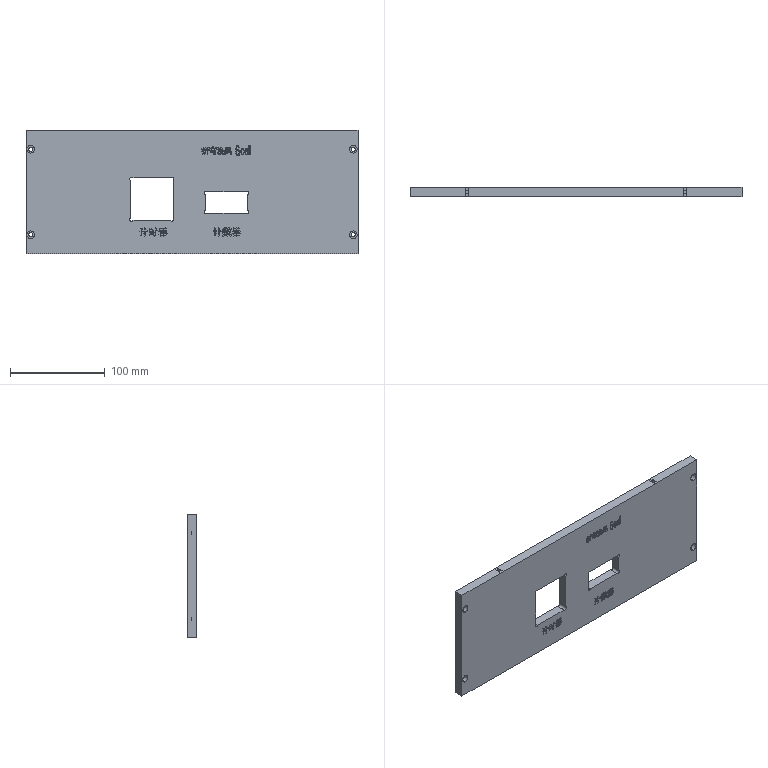Part | SolidWorks | features BaseBody 1, HoleWzd 1, ICE 1 | 1 solid | 961 faces | box 350 x 10 x 130 mm | volume 422656 mm3 | plane 925 | cylinder 36 | commonest cylinder face diameters 4 x12 4.2 x8 8 x8 3.3 x4 10 x4